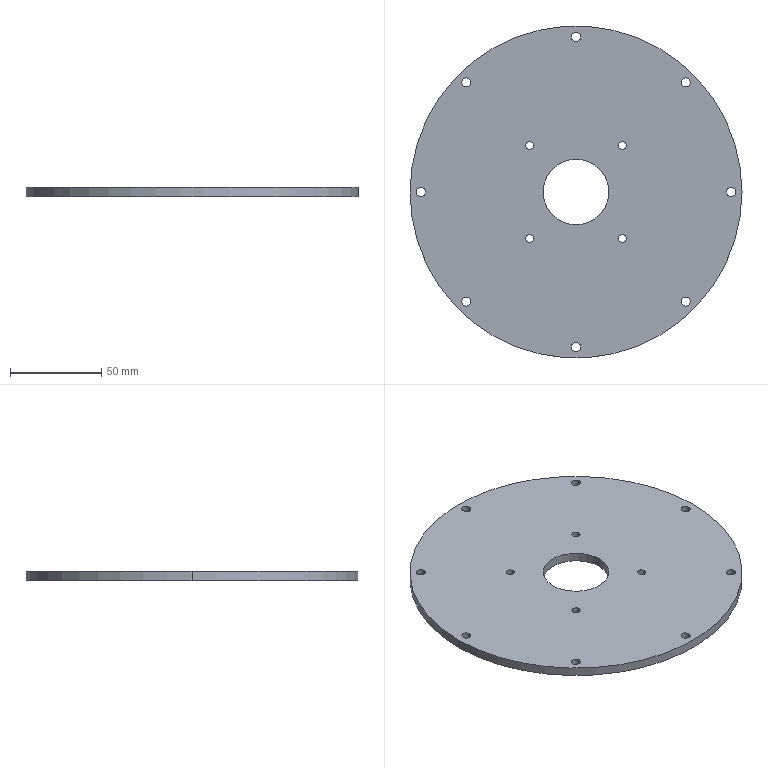Part | SolidWorks | features CirPattern 2, ICE 2, Extrusion 1 | 1 solid | 30 faces | box 182 x 182 x 5 mm | volume 123899 mm3 | cylinder 28 | plane 2 | commonest cylinder face diameters 5 x16 4.4 x8 36 x2 182 x2
STEP:
#1=CARTESIAN_POINT('',(-27.656,-25.456,2.5));
#2=VERTEX_POINT('',#1);
#3=CARTESIAN_POINT('',(-23.256,-25.456,2.5));
#4=VERTEX_POINT('',#3);
#5=CARTESIAN_POINT('',(-25.456,-25.456,2.5));
#6=DIRECTION('',(0.,0.,1.));
#7=DIRECTION('',(1.,0.,0.));
#8=AXIS2_PLACEMENT_3D('',#5,#6,#7);
#9=CIRCLE('',#8,2.2);
#10=EDGE_CURVE('',#2,#4,#9,.T.);
#11=ORIENTED_EDGE('',*,*,#10,.T.);
#12=CARTESIAN_POINT('',(-23.256,-25.456,-2.5));
#13=VERTEX_POINT('',#12);
#14=CARTESIAN_POINT('',(-23.256,-25.456,7.5));
#15=DIRECTION('',(0.,0.,-1.));
#16=VECTOR('',#15,1000.);
#17=LINE('',#14,#16);
#18=EDGE_CURVE('',#4,#13,#17,.T.);
#19=ORIENTED_EDGE('',*,*,#18,.T.);
#20=CARTESIAN_POINT('',(-27.656,-25.456,-2.5));
#21=VERTEX_POINT('',#20);
#22=CARTESIAN_POINT('',(-25.456,-25.456,-2.5));
#23=DIRECTION('',(0.,0.,-1.));
#24=DIRECTION('',(0.,-1.,0.));
#25=AXIS2_PLACEMENT_3D('',#22,#23,#24);
#26=CIRCLE('',#25,2.2);
#27=EDGE_CURVE('',#13,#21,#26,.T.);
#28=ORIENTED_EDGE('',*,*,#27,.T.);
#29=CARTESIAN_POINT('',(-27.656,-25.456,7.5));
#30=DIRECTION('',(0.,0.,-1.));
#31=VECTOR('',#30,1000.);
#32=LINE('',#29,#31);
#33=EDGE_CURVE('',#2,#21,#32,.T.);
#34=ORIENTED_EDGE('',*,*,#33,.F.);
#35=EDGE_LOOP('',(#11,#19,#28,#34));
#36=FACE_OUTER_BOUND('',#35,.T.);
#37=CARTESIAN_POINT('',(-25.456,-25.456,7.5));
#38=DIRECTION('',(0.,0.,-1.));
#39=DIRECTION('',(-1.,0.,0.));
#40=AXIS2_PLACEMENT_3D('',#37,#38,#39);
#41=CYLINDRICAL_SURFACE('',#40,2.2);
#42=ADVANCED_FACE('',(#36),#41,.F.);
#43=CARTESIAN_POINT('',(23.256,-25.456,2.5));
#44=VERTEX_POINT('',#43);
#45=CARTESIAN_POINT('',(27.656,-25.456,2.5));
#46=VERTEX_POINT('',#45);
#47=CARTESIAN_POINT('',(25.456,-25.456,2.5));
#48=DIRECTION('',(0.,0.,1.));
#49=DIRECTION('',(1.,0.,0.));
#50=AXIS2_PLACEMENT_3D('',#47,#48,#49);
#51=CIRCLE('',#50,2.2);
#52=EDGE_CURVE('',#44,#46,#51,.T.);
#53=ORIENTED_EDGE('',*,*,#52,.T.);
#54=CARTESIAN_POINT('',(27.656,-25.456,-2.5));
#55=VERTEX_POINT('',#54);
#56=CARTESIAN_POINT('',(27.656,-25.456,7.5));
#57=DIRECTION('',(0.,0.,-1.));
#58=VECTOR('',#57,1000.);
#59=LINE('',#56,#58);
#60=EDGE_CURVE('',#46,#55,#59,.T.);
#61=ORIENTED_EDGE('',*,*,#60,.T.);
#62=CARTESIAN_POINT('',(23.256,-25.456,-2.5));
#63=VERTEX_POINT('',#62);
#64=CARTESIAN_POINT('',(25.456,-25.456,-2.5));
#65=DIRECTION('',(0.,0.,-1.));
#66=DIRECTION('',(1.,0.,0.));
#67=AXIS2_PLACEMENT_3D('',#64,#65,#66);
#68=CIRCLE('',#67,2.2);
#69=EDGE_CURVE('',#55,#63,#68,.T.);
#70=ORIENTED_EDGE('',*,*,#69,.T.);
#71=CARTESIAN_POINT('',(23.256,-25.456,7.5));
#72=DIRECTION('',(0.,0.,-1.));
#73=VECTOR('',#72,1000.);
#74=LINE('',#71,#73);
#75=EDGE_CURVE('',#44,#63,#74,.T.);
#76=ORIENTED_EDGE('',*,*,#75,.F.);
#77=EDGE_LOOP('',(#53,#61,#70,#76));
#78=FACE_OUTER_BOUND('',#77,.T.);
#79=CARTESIAN_POINT('',(25.456,-25.456,7.5));
#80=DIRECTION('',(0.,0.,-1.));
#81=DIRECTION('',(-1.,0.,0.));
#82=AXIS2_PLACEMENT_3D('',#79,#80,#81);
#83=CYLINDRICAL_SURFACE('',#82,2.2);
#84=ADVANCED_FACE('',(#78),#83,.F.);
#85=CARTESIAN_POINT('',(23.256,25.456,2.5));
#86=VERTEX_POINT('',#85);
#87=CARTESIAN_POINT('',(27.656,25.456,2.5));
#88=VERTEX_POINT('',#87);
#89=CARTESIAN_POINT('',(25.456,25.456,2.5));
#90=DIRECTION('',(0.,0.,1.));
#91=DIRECTION('',(1.,0.,0.));
#92=AXIS2_PLACEMENT_3D('',#89,#90,#91);
#93=CIRCLE('',#92,2.2);
#94=EDGE_CURVE('',#86,#88,#93,.T.);
#95=ORIENTED_EDGE('',*,*,#94,.T.);
#96=CARTESIAN_POINT('',(27.656,25.456,-2.5));
#97=VERTEX_POINT('',#96);
#98=CARTESIAN_POINT('',(27.656,25.456,7.5));
#99=DIRECTION('',(0.,0.,-1.));
#100=VECTOR('',#99,1000.);
#101=LINE('',#98,#100);
#102=EDGE_CURVE('',#88,#97,#101,.T.);
#103=ORIENTED_EDGE('',*,*,#102,.T.);
#104=CARTESIAN_POINT('',(23.256,25.456,-2.5));
#105=VERTEX_POINT('',#104);
#106=CARTESIAN_POINT('',(25.456,25.456,-2.5));
#107=DIRECTION('',(0.,0.,-1.));
#108=DIRECTION('',(0.,1.,0.));
#109=AXIS2_PLACEMENT_3D('',#106,#107,#108);
#110=CIRCLE('',#109,2.2);
#111=EDGE_CURVE('',#97,#105,#110,.T.);
#112=ORIENTED_EDGE('',*,*,#111,.T.);
#113=CARTESIAN_POINT('',(23.256,25.456,7.5));
#114=DIRECTION('',(0.,0.,-1.));
#115=VECTOR('',#114,1000.);
#116=LINE('',#113,#115);
#117=EDGE_CURVE('',#86,#105,#116,.T.);
#118=ORIENTED_EDGE('',*,*,#117,.F.);
#119=EDGE_LOOP('',(#95,#103,#112,#118));
#120=FACE_OUTER_BOUND('',#119,.T.);
#121=CARTESIAN_POINT('',(25.456,25.456,7.5));
#122=DIRECTION('',(0.,0.,-1.));
#123=DIRECTION('',(-1.,0.,0.));
#124=AXIS2_PLACEMENT_3D('',#121,#122,#123);
#125=CYLINDRICAL_SURFACE('',#124,2.2);
#126=ADVANCED_FACE('',(#120),#125,.F.);
#127=CARTESIAN_POINT('',(-27.656,25.456,2.5));
#128=VERTEX_POINT('',#127);
#129=CARTESIAN_POINT('',(-23.256,25.456,2.5));
#130=VERTEX_POINT('',#129);
#131=CARTESIAN_POINT('',(-25.456,25.456,2.5));
#132=DIRECTION('',(0.,0.,1.));
#133=DIRECTION('',(1.,0.,0.));
#134=AXIS2_PLACEMENT_3D('',#131,#132,#133);
#135=CIRCLE('',#134,2.2);
#136=EDGE_CURVE('',#128,#130,#135,.T.);
#137=ORIENTED_EDGE('',*,*,#136,.T.);
#138=CARTESIAN_POINT('',(-23.256,25.456,-2.5));
#139=VERTEX_POINT('',#138);
#140=CARTESIAN_POINT('',(-23.256,25.456,7.5));
#141=DIRECTION('',(0.,0.,-1.));
#142=VECTOR('',#141,1000.);
#143=LINE('',#140,#142);
#144=EDGE_CURVE('',#130,#139,#143,.T.);
#145=ORIENTED_EDGE('',*,*,#144,.T.);
#146=CARTESIAN_POINT('',(-27.656,25.456,-2.5));
#147=VERTEX_POINT('',#146);
#148=CARTESIAN_POINT('',(-25.456,25.456,-2.5));
#149=DIRECTION('',(0.,0.,-1.));
#150=DIRECTION('',(-1.,0.,0.));
#151=AXIS2_PLACEMENT_3D('',#148,#149,#150);
#152=CIRCLE('',#151,2.2);
#153=EDGE_CURVE('',#139,#147,#152,.T.);
#154=ORIENTED_EDGE('',*,*,#153,.T.);
#155=CARTESIAN_POINT('',(-27.656,25.456,7.5));
#156=DIRECTION('',(0.,0.,-1.));
#157=VECTOR('',#156,1000.);
#158=LINE('',#155,#157);
#159=EDGE_CURVE('',#128,#147,#158,.T.);
#160=ORIENTED_EDGE('',*,*,#159,.F.);
#161=EDGE_LOOP('',(#137,#145,#154,#160));
#162=FACE_OUTER_BOUND('',#161,.T.);
#163=CARTESIAN_POINT('',(-25.456,25.456,7.5));
#164=DIRECTION('',(0.,0.,-1.));
#165=DIRECTION('',(-1.,0.,0.));
#166=AXIS2_PLACEMENT_3D('',#163,#164,#165);
#167=CYLINDRICAL_SURFACE('',#166,2.2);
#168=ADVANCED_FACE('',(#162),#167,.F.);
#169=CARTESIAN_POINT('',(-87.5,0.,-2.5));
#170=VERTEX_POINT('',#169);
#171=CARTESIAN_POINT('',(-82.5,0.,-2.5));
#172=VERTEX_POINT('',#171);
#173=CARTESIAN_POINT('',(-85.,0.,-2.5));
#174=DIRECTION('',(0.,0.,1.));
#175=DIRECTION('',(0.,1.,0.));
#176=AXIS2_PLACEMENT_3D('',#173,#174,#175);
#177=CIRCLE('',#176,2.5);
#178=EDGE_CURVE('',#170,#172,#177,.T.);
#179=ORIENTED_EDGE('',*,*,#178,.F.);
#180=CARTESIAN_POINT('',(-87.5,0.,2.5));
#181=VERTEX_POINT('',#180);
#182=CARTESIAN_POINT('',(-87.5,0.,-2.5));
#183=DIRECTION('',(0.,0.,1.));
#184=VECTOR('',#183,1000.);
#185=LINE('',#182,#184);
#186=EDGE_CURVE('',#170,#181,#185,.T.);
#187=ORIENTED_EDGE('',*,*,#186,.T.);
#188=CARTESIAN_POINT('',(-82.5,0.,2.5));
#189=VERTEX_POINT('',#188);
#190=CARTESIAN_POINT('',(-85.,0.,2.5));
#191=DIRECTION('',(0.,0.,1.));
#192=DIRECTION('',(0.,1.,0.));
#193=AXIS2_PLACEMENT_3D('',#190,#191,#192);
#194=CIRCLE('',#193,2.5);
#195=EDGE_CURVE('',#181,#189,#194,.T.);
#196=ORIENTED_EDGE('',*,*,#195,.T.);
#197=CARTESIAN_POINT('',(-82.5,0.,-2.5));
#198=DIRECTION('',(0.,0.,1.));
#199=VECTOR('',#198,1000.);
#200=LINE('',#197,#199);
#201=EDGE_CURVE('',#172,#189,#200,.T.);
#202=ORIENTED_EDGE('',*,*,#201,.F.);
#203=EDGE_LOOP('',(#179,#187,#196,#202));
#204=FACE_OUTER_BOUND('',#203,.T.);
#205=CARTESIAN_POINT('',(-85.,0.,-2.5));
#206=DIRECTION('',(0.,0.,1.));
#207=DIRECTION('',(1.,0.,0.));
#208=AXIS2_PLACEMENT_3D('',#205,#206,#207);
#209=CYLINDRICAL_SURFACE('',#208,2.5);
#210=ADVANCED_FACE('',(#204),#209,.F.);
#211=CARTESIAN_POINT('',(-62.604,-60.104,-2.5));
#212=VERTEX_POINT('',#211);
#213=CARTESIAN_POINT('',(-57.604,-60.104,-2.5));
#214=VERTEX_POINT('',#213);
#215=CARTESIAN_POINT('',(-60.104,-60.104,-2.5));
#216=DIRECTION('',(0.,0.,1.));
#217=DIRECTION('',(-0.7071,0.7071,0.));
#218=AXIS2_PLACEMENT_3D('',#215,#216,#217);
#219=CIRCLE('',#218,2.5);
#220=EDGE_CURVE('',#212,#214,#219,.T.);
#221=ORIENTED_EDGE('',*,*,#220,.F.);
#222=CARTESIAN_POINT('',(-62.604,-60.104,2.5));
#223=VERTEX_POINT('',#222);
#224=CARTESIAN_POINT('',(-62.604,-60.104,-2.5));
#225=DIRECTION('',(0.,0.,1.));
#226=VECTOR('',#225,1000.);
#227=LINE('',#224,#226);
#228=EDGE_CURVE('',#212,#223,#227,.T.);
#229=ORIENTED_EDGE('',*,*,#228,.T.);
#230=CARTESIAN_POINT('',(-57.604,-60.104,2.5));
#231=VERTEX_POINT('',#230);
#232=CARTESIAN_POINT('',(-60.104,-60.104,2.5));
#233=DIRECTION('',(0.,0.,1.));
#234=DIRECTION('',(-0.7071,0.7071,0.));
#235=AXIS2_PLACEMENT_3D('',#232,#233,#234);
#236=CIRCLE('',#235,2.5);
#237=EDGE_CURVE('',#223,#231,#236,.T.);
#238=ORIENTED_EDGE('',*,*,#237,.T.);
#239=CARTESIAN_POINT('',(-57.604,-60.104,-2.5));
#240=DIRECTION('',(0.,0.,1.));
#241=VECTOR('',#240,1000.);
#242=LINE('',#239,#241);
#243=EDGE_CURVE('',#214,#231,#242,.T.);
#244=ORIENTED_EDGE('',*,*,#243,.F.);
#245=EDGE_LOOP('',(#221,#229,#238,#244));
#246=FACE_OUTER_BOUND('',#245,.T.);
#247=CARTESIAN_POINT('',(-60.104,-60.104,-2.5));
#248=DIRECTION('',(0.,0.,1.));
#249=DIRECTION('',(1.,0.,0.));
#250=AXIS2_PLACEMENT_3D('',#247,#248,#249);
#251=CYLINDRICAL_SURFACE('',#250,2.5);
#252=ADVANCED_FACE('',(#246),#251,.F.);
#253=CARTESIAN_POINT('',(-2.5,-85.,-2.5));
#254=VERTEX_POINT('',#253);
#255=CARTESIAN_POINT('',(2.5,-85.,-2.5));
#256=VERTEX_POINT('',#255);
#257=CARTESIAN_POINT('',(0.,-85.,-2.5));
#258=DIRECTION('',(0.,0.,1.));
#259=DIRECTION('',(-1.,0.,0.));
#260=AXIS2_PLACEMENT_3D('',#257,#258,#259);
#261=CIRCLE('',#260,2.5);
#262=EDGE_CURVE('',#254,#256,#261,.T.);
#263=ORIENTED_EDGE('',*,*,#262,.F.);
#264=CARTESIAN_POINT('',(-2.5,-85.,2.5));
#265=VERTEX_POINT('',#264);
#266=CARTESIAN_POINT('',(-2.5,-85.,-2.5));
#267=DIRECTION('',(0.,0.,1.));
#268=VECTOR('',#267,1000.);
#269=LINE('',#266,#268);
#270=EDGE_CURVE('',#254,#265,#269,.T.);
#271=ORIENTED_EDGE('',*,*,#270,.T.);
#272=CARTESIAN_POINT('',(2.5,-85.,2.5));
#273=VERTEX_POINT('',#272);
#274=CARTESIAN_POINT('',(0.,-85.,2.5));
#275=DIRECTION('',(0.,0.,1.));
#276=DIRECTION('',(-1.,0.,0.));
#277=AXIS2_PLACEMENT_3D('',#274,#275,#276);
#278=CIRCLE('',#277,2.5);
#279=EDGE_CURVE('',#265,#273,#278,.T.);
#280=ORIENTED_EDGE('',*,*,#279,.T.);
#281=CARTESIAN_POINT('',(2.5,-85.,-2.5));
#282=DIRECTION('',(0.,0.,1.));
#283=VECTOR('',#282,1000.);
#284=LINE('',#281,#283);
#285=EDGE_CURVE('',#256,#273,#284,.T.);
#286=ORIENTED_EDGE('',*,*,#285,.F.);
#287=EDGE_LOOP('',(#263,#271,#280,#286));
#288=FACE_OUTER_BOUND('',#287,.T.);
#289=CARTESIAN_POINT('',(0.,-85.,-2.5));
#290=DIRECTION('',(0.,0.,1.));
#291=DIRECTION('',(1.,0.,0.));
#292=AXIS2_PLACEMENT_3D('',#289,#290,#291);
#293=CYLINDRICAL_SURFACE('',#292,2.5);
#294=ADVANCED_FACE('',(#288),#293,.F.);
#295=CARTESIAN_POINT('',(57.604,-60.104,-2.5));
#296=VERTEX_POINT('',#295);
#297=CARTESIAN_POINT('',(62.604,-60.104,-2.5));
#298=VERTEX_POINT('',#297);
#299=CARTESIAN_POINT('',(60.104,-60.104,-2.5));
#300=DIRECTION('',(0.,0.,1.));
#301=DIRECTION('',(-0.7071,-0.7071,0.));
#302=AXIS2_PLACEMENT_3D('',#299,#300,#301);
#303=CIRCLE('',#302,2.5);
#304=EDGE_CURVE('',#296,#298,#303,.T.);
#305=ORIENTED_EDGE('',*,*,#304,.F.);
#306=CARTESIAN_POINT('',(57.604,-60.104,2.5));
#307=VERTEX_POINT('',#306);
#308=CARTESIAN_POINT('',(57.604,-60.104,-2.5));
#309=DIRECTION('',(0.,0.,1.));
#310=VECTOR('',#309,1000.);
#311=LINE('',#308,#310);
#312=EDGE_CURVE('',#296,#307,#311,.T.);
#313=ORIENTED_EDGE('',*,*,#312,.T.);
#314=CARTESIAN_POINT('',(62.604,-60.104,2.5));
#315=VERTEX_POINT('',#314);
#316=CARTESIAN_POINT('',(60.104,-60.104,2.5));
#317=DIRECTION('',(0.,0.,1.));
#318=DIRECTION('',(-0.7071,-0.7071,0.));
#319=AXIS2_PLACEMENT_3D('',#316,#317,#318);
#320=CIRCLE('',#319,2.5);
#321=EDGE_CURVE('',#307,#315,#320,.T.);
#322=ORIENTED_EDGE('',*,*,#321,.T.);
#323=CARTESIAN_POINT('',(62.604,-60.104,-2.5));
#324=DIRECTION('',(0.,0.,1.));
#325=VECTOR('',#324,1000.);
#326=LINE('',#323,#325);
#327=EDGE_CURVE('',#298,#315,#326,.T.);
#328=ORIENTED_EDGE('',*,*,#327,.F.);
#329=EDGE_LOOP('',(#305,#313,#322,#328));
#330=FACE_OUTER_BOUND('',#329,.T.);
#331=CARTESIAN_POINT('',(60.104,-60.104,-2.5));
#332=DIRECTION('',(0.,0.,1.));
#333=DIRECTION('',(1.,0.,0.));
#334=AXIS2_PLACEMENT_3D('',#331,#332,#333);
#335=CYLINDRICAL_SURFACE('',#334,2.5);
#336=ADVANCED_FACE('',(#330),#335,.F.);
#337=CARTESIAN_POINT('',(82.5,0.,-2.5));
#338=VERTEX_POINT('',#337);
#339=CARTESIAN_POINT('',(87.5,0.,-2.5));
#340=VERTEX_POINT('',#339);
#341=CARTESIAN_POINT('',(85.,0.,-2.5));
#342=DIRECTION('',(0.,0.,1.));
#343=DIRECTION('',(0.,-1.,0.));
#344=AXIS2_PLACEMENT_3D('',#341,#342,#343);
#345=CIRCLE('',#344,2.5);
#346=EDGE_CURVE('',#338,#340,#345,.T.);
#347=ORIENTED_EDGE('',*,*,#346,.F.);
#348=CARTESIAN_POINT('',(82.5,0.,2.5));
#349=VERTEX_POINT('',#348);
#350=CARTESIAN_POINT('',(82.5,0.,-2.5));
#351=DIRECTION('',(0.,0.,1.));
#352=VECTOR('',#351,1000.);
#353=LINE('',#350,#352);
#354=EDGE_CURVE('',#338,#349,#353,.T.);
#355=ORIENTED_EDGE('',*,*,#354,.T.);
#356=CARTESIAN_POINT('',(87.5,0.,2.5));
#357=VERTEX_POINT('',#356);
#358=CARTESIAN_POINT('',(85.,0.,2.5));
#359=DIRECTION('',(0.,0.,1.));
#360=DIRECTION('',(0.,-1.,0.));
#361=AXIS2_PLACEMENT_3D('',#358,#359,#360);
#362=CIRCLE('',#361,2.5);
#363=EDGE_CURVE('',#349,#357,#362,.T.);
#364=ORIENTED_EDGE('',*,*,#363,.T.);
#365=CARTESIAN_POINT('',(87.5,0.,-2.5));
#366=DIRECTION('',(0.,0.,1.));
#367=VECTOR('',#366,1000.);
#368=LINE('',#365,#367);
#369=EDGE_CURVE('',#340,#357,#368,.T.);
#370=ORIENTED_EDGE('',*,*,#369,.F.);
#371=EDGE_LOOP('',(#347,#355,#364,#370));
#372=FACE_OUTER_BOUND('',#371,.T.);
#373=CARTESIAN_POINT('',(85.,0.,-2.5));
#374=DIRECTION('',(0.,0.,1.));
#375=DIRECTION('',(1.,0.,0.));
#376=AXIS2_PLACEMENT_3D('',#373,#374,#375);
#377=CYLINDRICAL_SURFACE('',#376,2.5);
#378=ADVANCED_FACE('',(#372),#377,.F.);
#379=CARTESIAN_POINT('',(57.604,60.104,-2.5));
#380=VERTEX_POINT('',#379);
#381=CARTESIAN_POINT('',(62.604,60.104,-2.5));
#382=VERTEX_POINT('',#381);
#383=CARTESIAN_POINT('',(60.104,60.104,-2.5));
#384=DIRECTION('',(0.,0.,1.));
#385=DIRECTION('',(0.7071,-0.7071,0.));
#386=AXIS2_PLACEMENT_3D('',#383,#384,#385);
#387=CIRCLE('',#386,2.5);
#388=EDGE_CURVE('',#380,#382,#387,.T.);
#389=ORIENTED_EDGE('',*,*,#388,.F.);
#390=CARTESIAN_POINT('',(57.604,60.104,2.5));
#391=VERTEX_POINT('',#390);
#392=CARTESIAN_POINT('',(57.604,60.104,-2.5));
#393=DIRECTION('',(0.,0.,1.));
#394=VECTOR('',#393,1000.);
#395=LINE('',#392,#394);
#396=EDGE_CURVE('',#380,#391,#395,.T.);
#397=ORIENTED_EDGE('',*,*,#396,.T.);
#398=CARTESIAN_POINT('',(62.604,60.104,2.5));
#399=VERTEX_POINT('',#398);
#400=CARTESIAN_POINT('',(60.104,60.104,2.5));
#401=DIRECTION('',(0.,0.,1.));
#402=DIRECTION('',(0.7071,-0.7071,0.));
#403=AXIS2_PLACEMENT_3D('',#400,#401,#402);
#404=CIRCLE('',#403,2.5);
#405=EDGE_CURVE('',#391,#399,#404,.T.);
#406=ORIENTED_EDGE('',*,*,#405,.T.);
#407=CARTESIAN_POINT('',(62.604,60.104,-2.5));
#408=DIRECTION('',(0.,0.,1.));
#409=VECTOR('',#408,1000.);
#410=LINE('',#407,#409);
#411=EDGE_CURVE('',#382,#399,#410,.T.);
#412=ORIENTED_EDGE('',*,*,#411,.F.);
#413=EDGE_LOOP('',(#389,#397,#406,#412));
#414=FACE_OUTER_BOUND('',#413,.T.);
#415=CARTESIAN_POINT('',(60.104,60.104,-2.5));
#416=DIRECTION('',(0.,0.,1.));
#417=DIRECTION('',(1.,0.,0.));
#418=AXIS2_PLACEMENT_3D('',#415,#416,#417);
#419=CYLINDRICAL_SURFACE('',#418,2.5);
#420=ADVANCED_FACE('',(#414),#419,.F.);
#421=CARTESIAN_POINT('',(-62.604,60.104,-2.5));
#422=VERTEX_POINT('',#421);
#423=CARTESIAN_POINT('',(-57.604,60.104,-2.5));
#424=VERTEX_POINT('',#423);
#425=CARTESIAN_POINT('',(-60.104,60.104,-2.5));
#426=DIRECTION('',(0.,0.,1.));
#427=DIRECTION('',(0.7071,0.7071,0.));
#428=AXIS2_PLACEMENT_3D('',#425,#426,#427);
#429=CIRCLE('',#428,2.5);
#430=EDGE_CURVE('',#422,#424,#429,.T.);
#431=ORIENTED_EDGE('',*,*,#430,.F.);
#432=CARTESIAN_POINT('',(-62.604,60.104,2.5));
#433=VERTEX_POINT('',#432);
#434=CARTESIAN_POINT('',(-62.604,60.104,-2.5));
#435=DIRECTION('',(0.,0.,1.));
#436=VECTOR('',#435,1000.);
#437=LINE('',#434,#436);
#438=EDGE_CURVE('',#422,#433,#437,.T.);
#439=ORIENTED_EDGE('',*,*,#438,.T.);
#440=CARTESIAN_POINT('',(-57.604,60.104,2.5));
#441=VERTEX_POINT('',#440);
#442=CARTESIAN_POINT('',(-60.104,60.104,2.5));
#443=DIRECTION('',(0.,0.,1.));
#444=DIRECTION('',(0.7071,0.7071,0.));
#445=AXIS2_PLACEMENT_3D('',#442,#443,#444);
#446=CIRCLE('',#445,2.5);
#447=EDGE_CURVE('',#433,#441,#446,.T.);
#448=ORIENTED_EDGE('',*,*,#447,.T.);
#449=CARTESIAN_POINT('',(-57.604,60.104,-2.5));
#450=DIRECTION('',(0.,0.,1.));
#451=VECTOR('',#450,1000.);
#452=LINE('',#449,#451);
#453=EDGE_CURVE('',#424,#441,#452,.T.);
#454=ORIENTED_EDGE('',*,*,#453,.F.);
#455=EDGE_LOOP('',(#431,#439,#448,#454));
#456=FACE_OUTER_BOUND('',#455,.T.);
#457=CARTESIAN_POINT('',(-60.104,60.104,-2.5));
#458=DIRECTION('',(0.,0.,1.));
#459=DIRECTION('',(1.,0.,0.));
#460=AXIS2_PLACEMENT_3D('',#457,#458,#459);
#461=CYLINDRICAL_SURFACE('',#460,2.5);
#462=ADVANCED_FACE('',(#456),#461,.F.);
#463=CARTESIAN_POINT('',(-2.5,85.,-2.5));
#464=VERTEX_POINT('',#463);
#465=CARTESIAN_POINT('',(2.5,85.,-2.5));
#466=VERTEX_POINT('',#465);
#467=CARTESIAN_POINT('',(0.,85.,-2.5));
#468=DIRECTION('',(0.,0.,1.));
#469=DIRECTION('',(1.,0.,0.));
#470=AXIS2_PLACEMENT_3D('',#467,#468,#469);
#471=CIRCLE('',#470,2.5);
#472=EDGE_CURVE('',#464,#466,#471,.T.);
#473=ORIENTED_EDGE('',*,*,#472,.F.);
#474=CARTESIAN_POINT('',(-2.5,85.,2.5));
#475=VERTEX_POINT('',#474);
#476=CARTESIAN_POINT('',(-2.5,85.,-2.5));
#477=DIRECTION('',(0.,0.,1.));
#478=VECTOR('',#477,1000.);
#479=LINE('',#476,#478);
#480=EDGE_CURVE('',#464,#475,#479,.T.);
#481=ORIENTED_EDGE('',*,*,#480,.T.);
#482=CARTESIAN_POINT('',(2.5,85.,2.5));
#483=VERTEX_POINT('',#482);
#484=CARTESIAN_POINT('',(0.,85.,2.5));
#485=DIRECTION('',(0.,0.,1.));
#486=DIRECTION('',(1.,0.,0.));
#487=AXIS2_PLACEMENT_3D('',#484,#485,#486);
#488=CIRCLE('',#487,2.5);
#489=EDGE_CURVE('',#475,#483,#488,.T.);
#490=ORIENTED_EDGE('',*,*,#489,.T.);
#491=CARTESIAN_POINT('',(2.5,85.,-2.5));
#492=DIRECTION('',(0.,0.,1.));
#493=VECTOR('',#492,1000.);
#494=LINE('',#491,#493);
#495=EDGE_CURVE('',#466,#483,#494,.T.);
#496=ORIENTED_EDGE('',*,*,#495,.F.);
#497=EDGE_LOOP('',(#473,#481,#490,#496));
#498=FACE_OUTER_BOUND('',#497,.T.);
#499=CARTESIAN_POINT('',(0.,85.,-2.5));
#500=DIRECTION('',(0.,0.,1.));
#501=DIRECTION('',(1.,0.,0.));
#502=AXIS2_PLACEMENT_3D('',#499,#500,#501);
#503=CYLINDRICAL_SURFACE('',#502,2.5);
#504=ADVANCED_FACE('',(#498),#503,.F.);
#505=CARTESIAN_POINT('',(-18.,0.,2.5));
#506=VERTEX_POINT('',#505);
#507=CARTESIAN_POINT('',(18.,0.,2.5));
#508=VERTEX_POINT('',#507);
#509=CARTESIAN_POINT('',(0.,0.,2.5));
#510=DIRECTION('',(0.,0.,1.));
#511=DIRECTION('',(1.,0.,0.));
#512=AXIS2_PLACEMENT_3D('',#509,#510,#511);
#513=CIRCLE('',#512,18.);
#514=EDGE_CURVE('',#506,#508,#513,.T.);
#515=ORIENTED_EDGE('',*,*,#514,.T.);
#516=CARTESIAN_POINT('',(18.,0.,-2.5));
#517=VERTEX_POINT('',#516);
#518=CARTESIAN_POINT('',(18.,0.,2.5));
#519=DIRECTION('',(0.,0.,-1.));
#520=VECTOR('',#519,1000.);
#521=LINE('',#518,#520);
#522=EDGE_CURVE('',#508,#517,#521,.T.);
#523=ORIENTED_EDGE('',*,*,#522,.T.);
#524=CARTESIAN_POINT('',(-18.,0.,-2.5));
#525=VERTEX_POINT('',#524);
#526=CARTESIAN_POINT('',(0.,0.,-2.5));
#527=DIRECTION('',(0.,0.,1.));
#528=DIRECTION('',(1.,0.,0.));
#529=AXIS2_PLACEMENT_3D('',#526,#527,#528);
#530=CIRCLE('',#529,18.);
#531=EDGE_CURVE('',#525,#517,#530,.T.);
#532=ORIENTED_EDGE('',*,*,#531,.F.);
#533=CARTESIAN_POINT('',(-18.,0.,2.5));
#534=DIRECTION('',(0.,0.,-1.));
#535=VECTOR('',#534,1000.);
#536=LINE('',#533,#535);
#537=EDGE_CURVE('',#506,#525,#536,.T.);
#538=ORIENTED_EDGE('',*,*,#537,.F.);
#539=EDGE_LOOP('',(#515,#523,#532,#538));
#540=FACE_OUTER_BOUND('',#539,.T.);
#541=CARTESIAN_POINT('',(0.,0.,2.5));
#542=DIRECTION('',(0.,0.,-1.));
#543=DIRECTION('',(-1.,0.,0.));
#544=AXIS2_PLACEMENT_3D('',#541,#542,#543);
#545=CYLINDRICAL_SURFACE('',#544,18.);
#546=ADVANCED_FACE('',(#540),#545,.F.);
#547=CARTESIAN_POINT('',(91.,0.,2.5));
#548=VERTEX_POINT('',#547);
#549=CARTESIAN_POINT('',(-91.,0.,2.5));
#550=VERTEX_POINT('',#549);
#551=CARTESIAN_POINT('',(0.,0.,2.5));
#552=DIRECTION('',(0.,0.,1.));
#553=DIRECTION('',(1.,0.,0.));
#554=AXIS2_PLACEMENT_3D('',#551,#552,#553);
#555=CIRCLE('',#554,91.);
#556=EDGE_CURVE('',#548,#550,#555,.T.);
#557=ORIENTED_EDGE('',*,*,#556,.F.);
#558=CARTESIAN_POINT('',(91.,0.,-2.5));
#559=VERTEX_POINT('',#558);
#560=CARTESIAN_POINT('',(91.,0.,2.5));
#561=DIRECTION('',(0.,0.,-1.));
#562=VECTOR('',#561,1000.);
#563=LINE('',#560,#562);
#564=EDGE_CURVE('',#548,#559,#563,.T.);
#565=ORIENTED_EDGE('',*,*,#564,.T.);
#566=CARTESIAN_POINT('',(-91.,0.,-2.5));
#567=VERTEX_POINT('',#566);
#568=CARTESIAN_POINT('',(0.,0.,-2.5));
#569=DIRECTION('',(0.,0.,1.));
#570=DIRECTION('',(1.,0.,0.));
#571=AXIS2_PLACEMENT_3D('',#568,#569,#570);
#572=CIRCLE('',#571,91.);
#573=EDGE_CURVE('',#559,#567,#572,.T.);
#574=ORIENTED_EDGE('',*,*,#573,.T.);
#575=CARTESIAN_POINT('',(-91.,0.,2.5));
#576=DIRECTION('',(0.,0.,-1.));
#577=VECTOR('',#576,1000.);
#578=LINE('',#575,#577);
#579=EDGE_CURVE('',#550,#567,#578,.T.);
#580=ORIENTED_EDGE('',*,*,#579,.F.);
#581=EDGE_LOOP('',(#557,#565,#574,#580));
#582=FACE_OUTER_BOUND('',#581,.T.);
#583=CARTESIAN_POINT('',(0.,0.,2.5));
#584=DIRECTION('',(0.,0.,-1.));
#585=DIRECTION('',(-1.,0.,0.));
#586=AXIS2_PLACEMENT_3D('',#583,#584,#585);
#587=CYLINDRICAL_SURFACE('',#586,91.);
#588=ADVANCED_FACE('',(#582),#587,.T.);
#589=ORIENTED_EDGE('',*,*,#10,.F.);
#590=CARTESIAN_POINT('',(-25.456,-25.456,2.5));
#591=DIRECTION('',(0.,0.,1.));
#592=DIRECTION('',(1.,0.,0.));
#593=AXIS2_PLACEMENT_3D('',#590,#591,#592);
#594=CIRCLE('',#593,2.2);
#595=EDGE_CURVE('',#4,#2,#594,.T.);
#596=ORIENTED_EDGE('',*,*,#595,.F.);
#597=EDGE_LOOP('',(#589,#596));
#598=FACE_BOUND('',#597,.T.);
#599=ORIENTED_EDGE('',*,*,#52,.F.);
#600=CARTESIAN_POINT('',(25.456,-25.456,2.5));
#601=DIRECTION('',(0.,0.,1.));
#602=DIRECTION('',(1.,0.,0.));
#603=AXIS2_PLACEMENT_3D('',#600,#601,#602);
#604=CIRCLE('',#603,2.2);
#605=EDGE_CURVE('',#46,#44,#604,.T.);
#606=ORIENTED_EDGE('',*,*,#605,.F.);
#607=EDGE_LOOP('',(#599,#606));
#608=FACE_BOUND('',#607,.T.);
#609=ORIENTED_EDGE('',*,*,#94,.F.);
#610=CARTESIAN_POINT('',(25.456,25.456,2.5));
#611=DIRECTION('',(0.,0.,1.));
#612=DIRECTION('',(1.,0.,0.));
#613=AXIS2_PLACEMENT_3D('',#610,#611,#612);
#614=CIRCLE('',#613,2.2);
#615=EDGE_CURVE('',#88,#86,#614,.T.);
#616=ORIENTED_EDGE('',*,*,#615,.F.);
#617=EDGE_LOOP('',(#609,#616));
#618=FACE_BOUND('',#617,.T.);
#619=ORIENTED_EDGE('',*,*,#136,.F.);
#620=CARTESIAN_POINT('',(-25.456,25.456,2.5));
#621=DIRECTION('',(0.,0.,1.));
#622=DIRECTION('',(1.,0.,0.));
#623=AXIS2_PLACEMENT_3D('',#620,#621,#622);
#624=CIRCLE('',#623,2.2);
#625=EDGE_CURVE('',#130,#128,#624,.T.);
#626=ORIENTED_EDGE('',*,*,#625,.F.);
#627=EDGE_LOOP('',(#619,#626));
#628=FACE_BOUND('',#627,.T.);
#629=CARTESIAN_POINT('',(-85.,0.,2.5));
#630=DIRECTION('',(0.,0.,1.));
#631=DIRECTION('',(0.,1.,0.));
#632=AXIS2_PLACEMENT_3D('',#629,#630,#631);
#633=CIRCLE('',#632,2.5);
#634=EDGE_CURVE('',#189,#181,#633,.T.);
#635=ORIENTED_EDGE('',*,*,#634,.F.);
#636=ORIENTED_EDGE('',*,*,#195,.F.);
#637=EDGE_LOOP('',(#635,#636));
#638=FACE_BOUND('',#637,.T.);
#639=CARTESIAN_POINT('',(-60.104,-60.104,2.5));
#640=DIRECTION('',(0.,0.,1.));
#641=DIRECTION('',(-0.7071,0.7071,0.));
#642=AXIS2_PLACEMENT_3D('',#639,#640,#641);
#643=CIRCLE('',#642,2.5);
#644=EDGE_CURVE('',#231,#223,#643,.T.);
#645=ORIENTED_EDGE('',*,*,#644,.F.);
#646=ORIENTED_EDGE('',*,*,#237,.F.);
#647=EDGE_LOOP('',(#645,#646));
#648=FACE_BOUND('',#647,.T.);
#649=CARTESIAN_POINT('',(0.,-85.,2.5));
#650=DIRECTION('',(0.,0.,1.));
#651=DIRECTION('',(-1.,0.,0.));
#652=AXIS2_PLACEMENT_3D('',#649,#650,#651);
#653=CIRCLE('',#652,2.5);
#654=EDGE_CURVE('',#273,#265,#653,.T.);
#655=ORIENTED_EDGE('',*,*,#654,.F.);
#656=ORIENTED_EDGE('',*,*,#279,.F.);
#657=EDGE_LOOP('',(#655,#656));
#658=FACE_BOUND('',#657,.T.);
#659=CARTESIAN_POINT('',(60.104,-60.104,2.5));
#660=DIRECTION('',(0.,0.,1.));
#661=DIRECTION('',(-0.7071,-0.7071,0.));
#662=AXIS2_PLACEMENT_3D('',#659,#660,#661);
#663=CIRCLE('',#662,2.5);
#664=EDGE_CURVE('',#315,#307,#663,.T.);
#665=ORIENTED_EDGE('',*,*,#664,.F.);
#666=ORIENTED_EDGE('',*,*,#321,.F.);
#667=EDGE_LOOP('',(#665,#666));
#668=FACE_BOUND('',#667,.T.);
#669=CARTESIAN_POINT('',(85.,0.,2.5));
#670=DIRECTION('',(0.,0.,1.));
#671=DIRECTION('',(0.,-1.,0.));
#672=AXIS2_PLACEMENT_3D('',#669,#670,#671);
#673=CIRCLE('',#672,2.5);
#674=EDGE_CURVE('',#357,#349,#673,.T.);
#675=ORIENTED_EDGE('',*,*,#674,.F.);
#676=ORIENTED_EDGE('',*,*,#363,.F.);
#677=EDGE_LOOP('',(#675,#676));
#678=FACE_BOUND('',#677,.T.);
#679=CARTESIAN_POINT('',(60.104,60.104,2.5));
#680=DIRECTION('',(0.,0.,1.));
#681=DIRECTION('',(0.7071,-0.7071,0.));
#682=AXIS2_PLACEMENT_3D('',#679,#680,#681);
#683=CIRCLE('',#682,2.5);
#684=EDGE_CURVE('',#399,#391,#683,.T.);
#685=ORIENTED_EDGE('',*,*,#684,.F.);
#686=ORIENTED_EDGE('',*,*,#405,.F.);
#687=EDGE_LOOP('',(#685,#686));
#688=FACE_BOUND('',#687,.T.);
#689=CARTESIAN_POINT('',(-60.104,60.104,2.5));
#690=DIRECTION('',(0.,0.,1.));
#691=DIRECTION('',(0.7071,0.7071,0.));
#692=AXIS2_PLACEMENT_3D('',#689,#690,#691);
#693=CIRCLE('',#692,2.5);
#694=EDGE_CURVE('',#441,#433,#693,.T.);
#695=ORIENTED_EDGE('',*,*,#694,.F.);
#696=ORIENTED_EDGE('',*,*,#447,.F.);
#697=EDGE_LOOP('',(#695,#696));
#698=FACE_BOUND('',#697,.T.);
#699=CARTESIAN_POINT('',(0.,85.,2.5));
#700=DIRECTION('',(0.,0.,1.));
#701=DIRECTION('',(1.,0.,0.));
#702=AXIS2_PLACEMENT_3D('',#699,#700,#701);
#703=CIRCLE('',#702,2.5);
#704=EDGE_CURVE('',#483,#475,#703,.T.);
#705=ORIENTED_EDGE('',*,*,#704,.F.);
#706=ORIENTED_EDGE('',*,*,#489,.F.);
#707=EDGE_LOOP('',(#705,#706));
#708=FACE_BOUND('',#707,.T.);
#709=CARTESIAN_POINT('',(0.,0.,2.5));
#710=DIRECTION('',(0.,0.,1.));
#711=DIRECTION('',(1.,0.,0.));
#712=AXIS2_PLACEMENT_3D('',#709,#710,#711);
#713=CIRCLE('',#712,91.);
#714=EDGE_CURVE('',#550,#548,#713,.T.);
#715=ORIENTED_EDGE('',*,*,#714,.T.);
#716=ORIENTED_EDGE('',*,*,#556,.T.);
#717=EDGE_LOOP('',(#715,#716));
#718=FACE_OUTER_BOUND('',#717,.T.);
#719=ORIENTED_EDGE('',*,*,#514,.F.);
#720=CARTESIAN_POINT('',(0.,0.,2.5));
#721=DIRECTION('',(0.,0.,1.));
#722=DIRECTION('',(1.,0.,0.));
#723=AXIS2_PLACEMENT_3D('',#720,#721,#722);
#724=CIRCLE('',#723,18.);
#725=EDGE_CURVE('',#508,#506,#724,.T.);
#726=ORIENTED_EDGE('',*,*,#725,.F.);
#727=EDGE_LOOP('',(#719,#726));
#728=FACE_BOUND('',#727,.T.);
#729=CARTESIAN_POINT('',(0.,0.,2.5));
#730=DIRECTION('',(0.,0.,1.));
#731=DIRECTION('',(1.,0.,0.));
#732=AXIS2_PLACEMENT_3D('',#729,#730,#731);
#733=PLANE('',#732);
#734=ADVANCED_FACE('',(#598,#608,#618,#628,#638,#648,#658,#668,#678,#688,#698,#708,#718,#728),#733,.T.);
#735=CARTESIAN_POINT('',(-25.456,-25.456,-2.5));
#736=DIRECTION('',(0.,0.,-1.));
#737=DIRECTION('',(0.,-1.,0.));
#738=AXIS2_PLACEMENT_3D('',#735,#736,#737);
#739=CIRCLE('',#738,2.2);
#740=EDGE_CURVE('',#21,#13,#739,.T.);
#741=ORIENTED_EDGE('',*,*,#740,.F.);
#742=ORIENTED_EDGE('',*,*,#27,.F.);
#743=EDGE_LOOP('',(#741,#742));
#744=FACE_BOUND('',#743,.T.);
#745=CARTESIAN_POINT('',(25.456,-25.456,-2.5));
#746=DIRECTION('',(0.,0.,-1.));
#747=DIRECTION('',(1.,0.,0.));
#748=AXIS2_PLACEMENT_3D('',#745,#746,#747);
#749=CIRCLE('',#748,2.2);
#750=EDGE_CURVE('',#63,#55,#749,.T.);
#751=ORIENTED_EDGE('',*,*,#750,.F.);
#752=ORIENTED_EDGE('',*,*,#69,.F.);
#753=EDGE_LOOP('',(#751,#752));
#754=FACE_BOUND('',#753,.T.);
#755=CARTESIAN_POINT('',(25.456,25.456,-2.5));
#756=DIRECTION('',(0.,0.,-1.));
#757=DIRECTION('',(0.,1.,0.));
#758=AXIS2_PLACEMENT_3D('',#755,#756,#757);
#759=CIRCLE('',#758,2.2);
#760=EDGE_CURVE('',#105,#97,#759,.T.);
#761=ORIENTED_EDGE('',*,*,#760,.F.);
#762=ORIENTED_EDGE('',*,*,#111,.F.);
#763=EDGE_LOOP('',(#761,#762));
#764=FACE_BOUND('',#763,.T.);
#765=CARTESIAN_POINT('',(-25.456,25.456,-2.5));
#766=DIRECTION('',(0.,0.,-1.));
#767=DIRECTION('',(-1.,0.,0.));
#768=AXIS2_PLACEMENT_3D('',#765,#766,#767);
#769=CIRCLE('',#768,2.2);
#770=EDGE_CURVE('',#147,#139,#769,.T.);
#771=ORIENTED_EDGE('',*,*,#770,.F.);
#772=ORIENTED_EDGE('',*,*,#153,.F.);
#773=EDGE_LOOP('',(#771,#772));
#774=FACE_BOUND('',#773,.T.);
#775=CARTESIAN_POINT('',(-85.,0.,-2.5));
#776=DIRECTION('',(0.,0.,1.));
#777=DIRECTION('',(0.,1.,0.));
#778=AXIS2_PLACEMENT_3D('',#775,#776,#777);
#779=CIRCLE('',#778,2.5);
#780=EDGE_CURVE('',#172,#170,#779,.T.);
#781=ORIENTED_EDGE('',*,*,#780,.T.);
#782=ORIENTED_EDGE('',*,*,#178,.T.);
#783=EDGE_LOOP('',(#781,#782));
#784=FACE_BOUND('',#783,.T.);
#785=CARTESIAN_POINT('',(-60.104,-60.104,-2.5));
#786=DIRECTION('',(0.,0.,1.));
#787=DIRECTION('',(-0.7071,0.7071,0.));
#788=AXIS2_PLACEMENT_3D('',#785,#786,#787);
#789=CIRCLE('',#788,2.5);
#790=EDGE_CURVE('',#214,#212,#789,.T.);
#791=ORIENTED_EDGE('',*,*,#790,.T.);
#792=ORIENTED_EDGE('',*,*,#220,.T.);
#793=EDGE_LOOP('',(#791,#792));
#794=FACE_BOUND('',#793,.T.);
#795=CARTESIAN_POINT('',(0.,-85.,-2.5));
#796=DIRECTION('',(0.,0.,1.));
#797=DIRECTION('',(-1.,0.,0.));
#798=AXIS2_PLACEMENT_3D('',#795,#796,#797);
#799=CIRCLE('',#798,2.5);
#800=EDGE_CURVE('',#256,#254,#799,.T.);
#801=ORIENTED_EDGE('',*,*,#800,.T.);
#802=ORIENTED_EDGE('',*,*,#262,.T.);
#803=EDGE_LOOP('',(#801,#802));
#804=FACE_BOUND('',#803,.T.);
#805=CARTESIAN_POINT('',(60.104,-60.104,-2.5));
#806=DIRECTION('',(0.,0.,1.));
#807=DIRECTION('',(-0.7071,-0.7071,0.));
#808=AXIS2_PLACEMENT_3D('',#805,#806,#807);
#809=CIRCLE('',#808,2.5);
#810=EDGE_CURVE('',#298,#296,#809,.T.);
#811=ORIENTED_EDGE('',*,*,#810,.T.);
#812=ORIENTED_EDGE('',*,*,#304,.T.);
#813=EDGE_LOOP('',(#811,#812));
#814=FACE_BOUND('',#813,.T.);
#815=CARTESIAN_POINT('',(85.,0.,-2.5));
#816=DIRECTION('',(0.,0.,1.));
#817=DIRECTION('',(0.,-1.,0.));
#818=AXIS2_PLACEMENT_3D('',#815,#816,#817);
#819=CIRCLE('',#818,2.5);
#820=EDGE_CURVE('',#340,#338,#819,.T.);
#821=ORIENTED_EDGE('',*,*,#820,.T.);
#822=ORIENTED_EDGE('',*,*,#346,.T.);
#823=EDGE_LOOP('',(#821,#822));
#824=FACE_BOUND('',#823,.T.);
#825=CARTESIAN_POINT('',(60.104,60.104,-2.5));
#826=DIRECTION('',(0.,0.,1.));
#827=DIRECTION('',(0.7071,-0.7071,0.));
#828=AXIS2_PLACEMENT_3D('',#825,#826,#827);
#829=CIRCLE('',#828,2.5);
#830=EDGE_CURVE('',#382,#380,#829,.T.);
#831=ORIENTED_EDGE('',*,*,#830,.T.);
#832=ORIENTED_EDGE('',*,*,#388,.T.);
#833=EDGE_LOOP('',(#831,#832));
#834=FACE_BOUND('',#833,.T.);
#835=CARTESIAN_POINT('',(-60.104,60.104,-2.5));
#836=DIRECTION('',(0.,0.,1.));
#837=DIRECTION('',(0.7071,0.7071,0.));
#838=AXIS2_PLACEMENT_3D('',#835,#836,#837);
#839=CIRCLE('',#838,2.5);
#840=EDGE_CURVE('',#424,#422,#839,.T.);
#841=ORIENTED_EDGE('',*,*,#840,.T.);
#842=ORIENTED_EDGE('',*,*,#430,.T.);
#843=EDGE_LOOP('',(#841,#842));
#844=FACE_BOUND('',#843,.T.);
#845=CARTESIAN_POINT('',(0.,85.,-2.5));
#846=DIRECTION('',(0.,0.,1.));
#847=DIRECTION('',(1.,0.,0.));
#848=AXIS2_PLACEMENT_3D('',#845,#846,#847);
#849=CIRCLE('',#848,2.5);
#850=EDGE_CURVE('',#466,#464,#849,.T.);
#851=ORIENTED_EDGE('',*,*,#850,.T.);
#852=ORIENTED_EDGE('',*,*,#472,.T.);
#853=EDGE_LOOP('',(#851,#852));
#854=FACE_BOUND('',#853,.T.);
#855=CARTESIAN_POINT('',(0.,0.,-2.5));
#856=DIRECTION('',(0.,0.,1.));
#857=DIRECTION('',(1.,0.,0.));
#858=AXIS2_PLACEMENT_3D('',#855,#856,#857);
#859=CIRCLE('',#858,91.);
#860=EDGE_CURVE('',#567,#559,#859,.T.);
#861=ORIENTED_EDGE('',*,*,#860,.F.);
#862=ORIENTED_EDGE('',*,*,#573,.F.);
#863=EDGE_LOOP('',(#861,#862));
#864=FACE_OUTER_BOUND('',#863,.T.);
#865=ORIENTED_EDGE('',*,*,#531,.T.);
#866=CARTESIAN_POINT('',(0.,0.,-2.5));
#867=DIRECTION('',(0.,0.,1.));
#868=DIRECTION('',(1.,0.,0.));
#869=AXIS2_PLACEMENT_3D('',#866,#867,#868);
#870=CIRCLE('',#869,18.);
#871=EDGE_CURVE('',#517,#525,#870,.T.);
#872=ORIENTED_EDGE('',*,*,#871,.T.);
#873=EDGE_LOOP('',(#865,#872));
#874=FACE_BOUND('',#873,.T.);
#875=CARTESIAN_POINT('',(0.,0.,-2.5));
#876=DIRECTION('',(0.,0.,1.));
#877=DIRECTION('',(1.,0.,0.));
#878=AXIS2_PLACEMENT_3D('',#875,#876,#877);
#879=PLANE('',#878);
#880=ADVANCED_FACE('',(#744,#754,#764,#774,#784,#794,#804,#814,#824,#834,#844,#854,#864,#874),#879,.F.);
#881=ORIENTED_EDGE('',*,*,#564,.F.);
#882=ORIENTED_EDGE('',*,*,#714,.F.);
#883=ORIENTED_EDGE('',*,*,#579,.T.);
#884=ORIENTED_EDGE('',*,*,#860,.T.);
#885=EDGE_LOOP('',(#881,#882,#883,#884));
#886=FACE_OUTER_BOUND('',#885,.T.);
#887=CARTESIAN_POINT('',(0.,0.,2.5));
#888=DIRECTION('',(0.,0.,-1.));
#889=DIRECTION('',(-1.,0.,0.));
#890=AXIS2_PLACEMENT_3D('',#887,#888,#889);
#891=CYLINDRICAL_SURFACE('',#890,91.);
#892=ADVANCED_FACE('',(#886),#891,.T.);
#893=ORIENTED_EDGE('',*,*,#522,.F.);
#894=ORIENTED_EDGE('',*,*,#725,.T.);
#895=ORIENTED_EDGE('',*,*,#537,.T.);
#896=ORIENTED_EDGE('',*,*,#871,.F.);
#897=EDGE_LOOP('',(#893,#894,#895,#896));
#898=FACE_OUTER_BOUND('',#897,.T.);
#899=CARTESIAN_POINT('',(0.,0.,2.5));
#900=DIRECTION('',(0.,0.,-1.));
#901=DIRECTION('',(-1.,0.,0.));
#902=AXIS2_PLACEMENT_3D('',#899,#900,#901);
#903=CYLINDRICAL_SURFACE('',#902,18.);
#904=ADVANCED_FACE('',(#898),#903,.F.);
#905=ORIENTED_EDGE('',*,*,#480,.F.);
#906=ORIENTED_EDGE('',*,*,#850,.F.);
#907=ORIENTED_EDGE('',*,*,#495,.T.);
#908=ORIENTED_EDGE('',*,*,#704,.T.);
#909=EDGE_LOOP('',(#905,#906,#907,#908));
#910=FACE_OUTER_BOUND('',#909,.T.);
#911=CARTESIAN_POINT('',(0.,85.,-2.5));
#912=DIRECTION('',(0.,0.,1.));
#913=DIRECTION('',(1.,0.,0.));
#914=AXIS2_PLACEMENT_3D('',#911,#912,#913);
#915=CYLINDRICAL_SURFACE('',#914,2.5);
#916=ADVANCED_FACE('',(#910),#915,.F.);
#917=ORIENTED_EDGE('',*,*,#438,.F.);
#918=ORIENTED_EDGE('',*,*,#840,.F.);
#919=ORIENTED_EDGE('',*,*,#453,.T.);
#920=ORIENTED_EDGE('',*,*,#694,.T.);
#921=EDGE_LOOP('',(#917,#918,#919,#920));
#922=FACE_OUTER_BOUND('',#921,.T.);
#923=CARTESIAN_POINT('',(-60.104,60.104,-2.5));
#924=DIRECTION('',(0.,0.,1.));
#925=DIRECTION('',(1.,0.,0.));
#926=AXIS2_PLACEMENT_3D('',#923,#924,#925);
#927=CYLINDRICAL_SURFACE('',#926,2.5);
#928=ADVANCED_FACE('',(#922),#927,.F.);
#929=ORIENTED_EDGE('',*,*,#396,.F.);
#930=ORIENTED_EDGE('',*,*,#830,.F.);
#931=ORIENTED_EDGE('',*,*,#411,.T.);
#932=ORIENTED_EDGE('',*,*,#684,.T.);
#933=EDGE_LOOP('',(#929,#930,#931,#932));
#934=FACE_OUTER_BOUND('',#933,.T.);
#935=CARTESIAN_POINT('',(60.104,60.104,-2.5));
#936=DIRECTION('',(0.,0.,1.));
#937=DIRECTION('',(1.,0.,0.));
#938=AXIS2_PLACEMENT_3D('',#935,#936,#937);
#939=CYLINDRICAL_SURFACE('',#938,2.5);
#940=ADVANCED_FACE('',(#934),#939,.F.);
#941=ORIENTED_EDGE('',*,*,#354,.F.);
#942=ORIENTED_EDGE('',*,*,#820,.F.);
#943=ORIENTED_EDGE('',*,*,#369,.T.);
#944=ORIENTED_EDGE('',*,*,#674,.T.);
#945=EDGE_LOOP('',(#941,#942,#943,#944));
#946=FACE_OUTER_BOUND('',#945,.T.);
#947=CARTESIAN_POINT('',(85.,0.,-2.5));
#948=DIRECTION('',(0.,0.,1.));
#949=DIRECTION('',(1.,0.,0.));
#950=AXIS2_PLACEMENT_3D('',#947,#948,#949);
#951=CYLINDRICAL_SURFACE('',#950,2.5);
#952=ADVANCED_FACE('',(#946),#951,.F.);
#953=ORIENTED_EDGE('',*,*,#312,.F.);
#954=ORIENTED_EDGE('',*,*,#810,.F.);
#955=ORIENTED_EDGE('',*,*,#327,.T.);
#956=ORIENTED_EDGE('',*,*,#664,.T.);
#957=EDGE_LOOP('',(#953,#954,#955,#956));
#958=FACE_OUTER_BOUND('',#957,.T.);
#959=CARTESIAN_POINT('',(60.104,-60.104,-2.5));
#960=DIRECTION('',(0.,0.,1.));
#961=DIRECTION('',(1.,0.,0.));
#962=AXIS2_PLACEMENT_3D('',#959,#960,#961);
#963=CYLINDRICAL_SURFACE('',#962,2.5);
#964=ADVANCED_FACE('',(#958),#963,.F.);
#965=ORIENTED_EDGE('',*,*,#270,.F.);
#966=ORIENTED_EDGE('',*,*,#800,.F.);
#967=ORIENTED_EDGE('',*,*,#285,.T.);
#968=ORIENTED_EDGE('',*,*,#654,.T.);
#969=EDGE_LOOP('',(#965,#966,#967,#968));
#970=FACE_OUTER_BOUND('',#969,.T.);
#971=CARTESIAN_POINT('',(0.,-85.,-2.5));
#972=DIRECTION('',(0.,0.,1.));
#973=DIRECTION('',(1.,0.,0.));
#974=AXIS2_PLACEMENT_3D('',#971,#972,#973);
#975=CYLINDRICAL_SURFACE('',#974,2.5);
#976=ADVANCED_FACE('',(#970),#975,.F.);
#977=ORIENTED_EDGE('',*,*,#228,.F.);
#978=ORIENTED_EDGE('',*,*,#790,.F.);
#979=ORIENTED_EDGE('',*,*,#243,.T.);
#980=ORIENTED_EDGE('',*,*,#644,.T.);
#981=EDGE_LOOP('',(#977,#978,#979,#980));
#982=FACE_OUTER_BOUND('',#981,.T.);
#983=CARTESIAN_POINT('',(-60.104,-60.104,-2.5));
#984=DIRECTION('',(0.,0.,1.));
#985=DIRECTION('',(1.,0.,0.));
#986=AXIS2_PLACEMENT_3D('',#983,#984,#985);
#987=CYLINDRICAL_SURFACE('',#986,2.5);
#988=ADVANCED_FACE('',(#982),#987,.F.);
#989=ORIENTED_EDGE('',*,*,#186,.F.);
#990=ORIENTED_EDGE('',*,*,#780,.F.);
#991=ORIENTED_EDGE('',*,*,#201,.T.);
#992=ORIENTED_EDGE('',*,*,#634,.T.);
#993=EDGE_LOOP('',(#989,#990,#991,#992));
#994=FACE_OUTER_BOUND('',#993,.T.);
#995=CARTESIAN_POINT('',(-85.,0.,-2.5));
#996=DIRECTION('',(0.,0.,1.));
#997=DIRECTION('',(1.,0.,0.));
#998=AXIS2_PLACEMENT_3D('',#995,#996,#997);
#999=CYLINDRICAL_SURFACE('',#998,2.5);
#1000=ADVANCED_FACE('',(#994),#999,.F.);
#1001=ORIENTED_EDGE('',*,*,#144,.F.);
#1002=ORIENTED_EDGE('',*,*,#625,.T.);
#1003=ORIENTED_EDGE('',*,*,#159,.T.);
#1004=ORIENTED_EDGE('',*,*,#770,.T.);
#1005=EDGE_LOOP('',(#1001,#1002,#1003,#1004));
#1006=FACE_OUTER_BOUND('',#1005,.T.);
#1007=CARTESIAN_POINT('',(-25.456,25.456,7.5));
#1008=DIRECTION('',(0.,0.,-1.));
#1009=DIRECTION('',(-1.,0.,0.));
#1010=AXIS2_PLACEMENT_3D('',#1007,#1008,#1009);
#1011=CYLINDRICAL_SURFACE('',#1010,2.2);
#1012=ADVANCED_FACE('',(#1006),#1011,.F.);
#1013=ORIENTED_EDGE('',*,*,#102,.F.);
#1014=ORIENTED_EDGE('',*,*,#615,.T.);
#1015=ORIENTED_EDGE('',*,*,#117,.T.);
#1016=ORIENTED_EDGE('',*,*,#760,.T.);
#1017=EDGE_LOOP('',(#1013,#1014,#1015,#1016));
#1018=FACE_OUTER_BOUND('',#1017,.T.);
#1019=CARTESIAN_POINT('',(25.456,25.456,7.5));
#1020=DIRECTION('',(0.,0.,-1.));
#1021=DIRECTION('',(-1.,0.,0.));
#1022=AXIS2_PLACEMENT_3D('',#1019,#1020,#1021);
#1023=CYLINDRICAL_SURFACE('',#1022,2.2);
#1024=ADVANCED_FACE('',(#1018),#1023,.F.);
#1025=ORIENTED_EDGE('',*,*,#60,.F.);
#1026=ORIENTED_EDGE('',*,*,#605,.T.);
#1027=ORIENTED_EDGE('',*,*,#75,.T.);
#1028=ORIENTED_EDGE('',*,*,#750,.T.);
#1029=EDGE_LOOP('',(#1025,#1026,#1027,#1028));
#1030=FACE_OUTER_BOUND('',#1029,.T.);
#1031=CARTESIAN_POINT('',(25.456,-25.456,7.5));
#1032=DIRECTION('',(0.,0.,-1.));
#1033=DIRECTION('',(-1.,0.,0.));
#1034=AXIS2_PLACEMENT_3D('',#1031,#1032,#1033);
#1035=CYLINDRICAL_SURFACE('',#1034,2.2);
#1036=ADVANCED_FACE('',(#1030),#1035,.F.);
#1037=ORIENTED_EDGE('',*,*,#18,.F.);
#1038=ORIENTED_EDGE('',*,*,#595,.T.);
#1039=ORIENTED_EDGE('',*,*,#33,.T.);
#1040=ORIENTED_EDGE('',*,*,#740,.T.);
#1041=EDGE_LOOP('',(#1037,#1038,#1039,#1040));
#1042=FACE_OUTER_BOUND('',#1041,.T.);
#1043=CARTESIAN_POINT('',(-25.456,-25.456,7.5));
#1044=DIRECTION('',(0.,0.,-1.));
#1045=DIRECTION('',(-1.,0.,0.));
#1046=AXIS2_PLACEMENT_3D('',#1043,#1044,#1045);
#1047=CYLINDRICAL_SURFACE('',#1046,2.2);
#1048=ADVANCED_FACE('',(#1042),#1047,.F.);
#1049=CLOSED_SHELL('',(#42,#84,#126,#168,#210,#252,#294,#336,#378,#420,#462,#504,#546,#588,#734,#880,#892,#904,#916,#928,#940,#952,#964,#976,#988,#1000,#1012,#1024,#1036,#1048));
#1050=MANIFOLD_SOLID_BREP('',#1049);
#1051=CARTESIAN_POINT('',(0.,0.,0.));
#1052=DIRECTION('',(0.,0.,1.));
#1053=DIRECTION('',(1.,0.,0.));
#1054=AXIS2_PLACEMENT_3D('',#1051,#1052,#1053);
#1055=(LENGTH_UNIT()NAMED_UNIT(*)SI_UNIT(.MILLI.,.METRE.));
#1056=UNCERTAINTY_MEASURE_WITH_UNIT(LENGTH_MEASURE(0.00001),#1055,'','');
#1057=(NAMED_UNIT(*)PLANE_ANGLE_UNIT()SI_UNIT($,.RADIAN.));
#1058=(NAMED_UNIT(*)SI_UNIT($,.STERADIAN.)SOLID_ANGLE_UNIT());
#1059=(GEOMETRIC_REPRESENTATION_CONTEXT(3)GLOBAL_UNCERTAINTY_ASSIGNED_CONTEXT((#1056))GLOBAL_UNIT_ASSIGNED_CONTEXT((#1055,#1057,#1058))REPRESENTATION_CONTEXT('',''));
#1060=ADVANCED_BREP_SHAPE_REPRESENTATION('',(#1050,#1054),#1059);